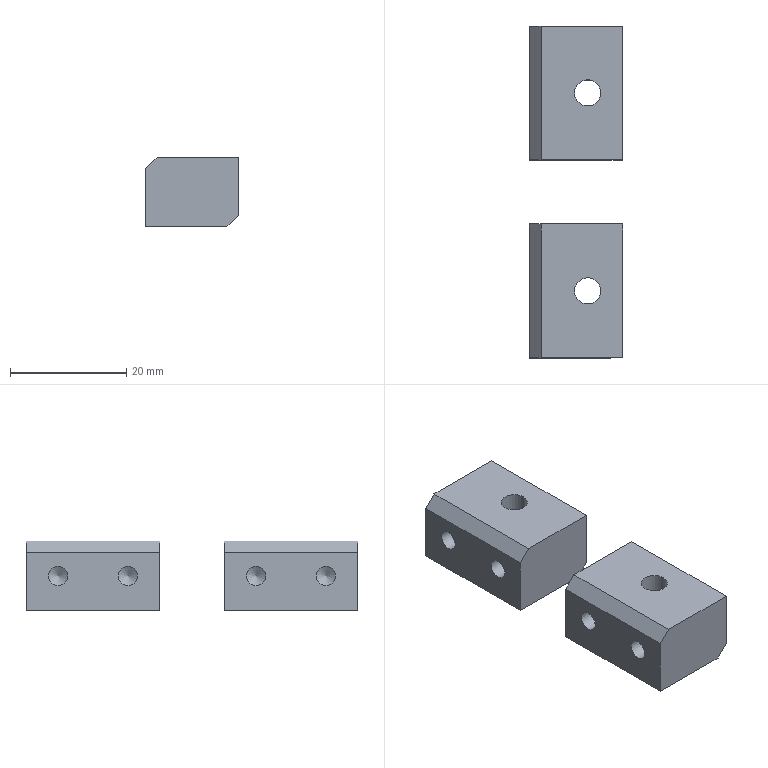Part | NX | 2 solids | 30 faces | box 16 x 57 x 12 mm | volume 7634 mm3 | plane 18 | cylinder 8 | cone 4 | commonest cylinder face diameters 3.3 x4 4.5 x2 8 x2
STEP:
#1=CARTESIAN_POINT('',(14.,11.5,-12.));
#2=VERTEX_POINT('',#1);
#3=CARTESIAN_POINT('',(10.,11.5,-12.));
#4=DIRECTION('',(0.,0.,-1.));
#5=DIRECTION('',(-1.,0.,0.));
#6=AXIS2_PLACEMENT_3D('',#3,#4,#5);
#7=CIRCLE('',#6,4.);
#8=EDGE_CURVE('',#2,#2,#7,.T.);
#9=ORIENTED_EDGE('',*,*,#8,.T.);
#10=EDGE_LOOP('',(#9));
#11=FACE_BOUND('',#10,.T.);
#12=CARTESIAN_POINT('',(6.,11.5,-7.));
#13=VERTEX_POINT('',#12);
#14=CARTESIAN_POINT('',(10.,11.5,-7.));
#15=DIRECTION('',(0.,0.,-1.));
#16=DIRECTION('',(-1.,0.,0.));
#17=AXIS2_PLACEMENT_3D('',#14,#15,#16);
#18=CIRCLE('',#17,4.);
#19=EDGE_CURVE('',#13,#13,#18,.T.);
#20=ORIENTED_EDGE('',*,*,#19,.F.);
#21=EDGE_LOOP('',(#20));
#22=FACE_BOUND('',#21,.T.);
#23=CARTESIAN_POINT('',(10.,11.5,-12.));
#24=DIRECTION('',(0.,0.,-1.));
#25=DIRECTION('',(-1.,0.,0.));
#26=AXIS2_PLACEMENT_3D('',#23,#24,#25);
#27=CYLINDRICAL_SURFACE('',#26,4.);
#28=ADVANCED_FACE('',(#11,#22),#27,.F.);
#29=ORIENTED_EDGE('',*,*,#19,.T.);
#30=EDGE_LOOP('',(#29));
#31=FACE_BOUND('',#30,.T.);
#32=CARTESIAN_POINT('',(7.75,11.5,-7.));
#33=VERTEX_POINT('',#32);
#34=CARTESIAN_POINT('',(10.,11.5,-7.));
#35=DIRECTION('',(0.,0.,-1.));
#36=DIRECTION('',(-1.,0.,0.));
#37=AXIS2_PLACEMENT_3D('',#34,#35,#36);
#38=CIRCLE('',#37,2.25);
#39=EDGE_CURVE('',#33,#33,#38,.T.);
#40=ORIENTED_EDGE('',*,*,#39,.F.);
#41=EDGE_LOOP('',(#40));
#42=FACE_BOUND('',#41,.T.);
#43=CARTESIAN_POINT('',(12.25,11.5,-7.));
#44=DIRECTION('',(0.,0.,1.));
#45=DIRECTION('',(1.,0.,0.));
#46=AXIS2_PLACEMENT_3D('',#43,#44,#45);
#47=PLANE('',#46);
#48=ADVANCED_FACE('',(#31,#42),#47,.F.);
#49=ORIENTED_EDGE('',*,*,#39,.T.);
#50=EDGE_LOOP('',(#49));
#51=FACE_BOUND('',#50,.T.);
#52=CARTESIAN_POINT('',(7.75,11.5,0.));
#53=VERTEX_POINT('',#52);
#54=CARTESIAN_POINT('',(10.,11.5,0.));
#55=DIRECTION('',(0.,0.,-1.));
#56=DIRECTION('',(-1.,0.,0.));
#57=AXIS2_PLACEMENT_3D('',#54,#55,#56);
#58=CIRCLE('',#57,2.25);
#59=EDGE_CURVE('',#53,#53,#58,.T.);
#60=ORIENTED_EDGE('',*,*,#59,.F.);
#61=EDGE_LOOP('',(#60));
#62=FACE_BOUND('',#61,.T.);
#63=CARTESIAN_POINT('',(10.,11.5,-12.));
#64=DIRECTION('',(0.,0.,-1.));
#65=DIRECTION('',(-1.,0.,0.));
#66=AXIS2_PLACEMENT_3D('',#63,#64,#65);
#67=CYLINDRICAL_SURFACE('',#66,2.25);
#68=ADVANCED_FACE('',(#51,#62),#67,.F.);
#69=CARTESIAN_POINT('',(0.,5.5,-4.35));
#70=VERTEX_POINT('',#69);
#71=CARTESIAN_POINT('',(0.,5.5,-6.));
#72=DIRECTION('',(-1.,0.,0.));
#73=DIRECTION('',(0.,0.,1.));
#74=AXIS2_PLACEMENT_3D('',#71,#72,#73);
#75=CIRCLE('',#74,1.65);
#76=EDGE_CURVE('',#70,#70,#75,.T.);
#77=ORIENTED_EDGE('',*,*,#76,.T.);
#78=EDGE_LOOP('',(#77));
#79=FACE_BOUND('',#78,.T.);
#80=CARTESIAN_POINT('',(8.1,5.5,-4.35));
#81=VERTEX_POINT('',#80);
#82=CARTESIAN_POINT('',(8.1,5.5,-6.));
#83=DIRECTION('',(-1.,0.,0.));
#84=DIRECTION('',(0.,0.,1.));
#85=AXIS2_PLACEMENT_3D('',#82,#83,#84);
#86=CIRCLE('',#85,1.65);
#87=EDGE_CURVE('',#81,#81,#86,.T.);
#88=ORIENTED_EDGE('',*,*,#87,.F.);
#89=EDGE_LOOP('',(#88));
#90=FACE_BOUND('',#89,.T.);
#91=CARTESIAN_POINT('',(0.,5.5,-6.));
#92=DIRECTION('',(-1.,0.,0.));
#93=DIRECTION('',(0.,0.,1.));
#94=AXIS2_PLACEMENT_3D('',#91,#92,#93);
#95=CYLINDRICAL_SURFACE('',#94,1.65);
#96=ADVANCED_FACE('',(#79,#90),#95,.F.);
#97=CARTESIAN_POINT('',(9.091,5.5,-6.));
#98=VERTEX_POINT('',#97);
#99=VERTEX_LOOP('',#98);
#100=FACE_BOUND('',#99,.T.);
#101=ORIENTED_EDGE('',*,*,#87,.T.);
#102=EDGE_LOOP('',(#101));
#103=FACE_BOUND('',#102,.T.);
#104=CARTESIAN_POINT('',(8.1,5.5,-6.));
#105=DIRECTION('',(-1.,0.,0.));
#106=DIRECTION('',(0.,0.,1.));
#107=AXIS2_PLACEMENT_3D('',#104,#105,#106);
#108=CONICAL_SURFACE('',#107,1.65,1.03);
#109=ADVANCED_FACE('',(#100,#103),#108,.F.);
#110=CARTESIAN_POINT('',(0.,17.5,-4.35));
#111=VERTEX_POINT('',#110);
#112=CARTESIAN_POINT('',(0.,17.5,-6.));
#113=DIRECTION('',(-1.,0.,0.));
#114=DIRECTION('',(0.,0.,1.));
#115=AXIS2_PLACEMENT_3D('',#112,#113,#114);
#116=CIRCLE('',#115,1.65);
#117=EDGE_CURVE('',#111,#111,#116,.T.);
#118=ORIENTED_EDGE('',*,*,#117,.T.);
#119=EDGE_LOOP('',(#118));
#120=FACE_BOUND('',#119,.T.);
#121=CARTESIAN_POINT('',(8.1,17.5,-4.35));
#122=VERTEX_POINT('',#121);
#123=CARTESIAN_POINT('',(8.1,17.5,-6.));
#124=DIRECTION('',(-1.,0.,0.));
#125=DIRECTION('',(0.,0.,1.));
#126=AXIS2_PLACEMENT_3D('',#123,#124,#125);
#127=CIRCLE('',#126,1.65);
#128=EDGE_CURVE('',#122,#122,#127,.T.);
#129=ORIENTED_EDGE('',*,*,#128,.F.);
#130=EDGE_LOOP('',(#129));
#131=FACE_BOUND('',#130,.T.);
#132=CARTESIAN_POINT('',(0.,17.5,-6.));
#133=DIRECTION('',(-1.,0.,0.));
#134=DIRECTION('',(0.,0.,1.));
#135=AXIS2_PLACEMENT_3D('',#132,#133,#134);
#136=CYLINDRICAL_SURFACE('',#135,1.65);
#137=ADVANCED_FACE('',(#120,#131),#136,.F.);
#138=CARTESIAN_POINT('',(9.091,17.5,-6.));
#139=VERTEX_POINT('',#138);
#140=VERTEX_LOOP('',#139);
#141=FACE_BOUND('',#140,.T.);
#142=ORIENTED_EDGE('',*,*,#128,.T.);
#143=EDGE_LOOP('',(#142));
#144=FACE_BOUND('',#143,.T.);
#145=CARTESIAN_POINT('',(8.1,17.5,-6.));
#146=DIRECTION('',(-1.,0.,0.));
#147=DIRECTION('',(0.,0.,1.));
#148=AXIS2_PLACEMENT_3D('',#145,#146,#147);
#149=CONICAL_SURFACE('',#148,1.65,1.03);
#150=ADVANCED_FACE('',(#141,#144),#149,.F.);
#151=CARTESIAN_POINT('',(0.,23.,-2.));
#152=VERTEX_POINT('',#151);
#153=CARTESIAN_POINT('',(2.,23.,0.));
#154=VERTEX_POINT('',#153);
#155=CARTESIAN_POINT('',(1.,23.,-1.));
#156=DIRECTION('',(0.7071,0.,0.7071));
#157=VECTOR('',#156,1000.);
#158=LINE('',#155,#157);
#159=EDGE_CURVE('',#152,#154,#158,.T.);
#160=ORIENTED_EDGE('',*,*,#159,.F.);
#161=CARTESIAN_POINT('',(0.,0.,-2.));
#162=VERTEX_POINT('',#161);
#163=CARTESIAN_POINT('',(0.,23.,-2.));
#164=DIRECTION('',(0.,1.,0.));
#165=VECTOR('',#164,1000.);
#166=LINE('',#163,#165);
#167=EDGE_CURVE('',#162,#152,#166,.T.);
#168=ORIENTED_EDGE('',*,*,#167,.F.);
#169=CARTESIAN_POINT('',(2.,0.,0.));
#170=VERTEX_POINT('',#169);
#171=CARTESIAN_POINT('',(2.,0.,0.));
#172=DIRECTION('',(-0.7071,0.,-0.7071));
#173=VECTOR('',#172,1000.);
#174=LINE('',#171,#173);
#175=EDGE_CURVE('',#170,#162,#174,.T.);
#176=ORIENTED_EDGE('',*,*,#175,.F.);
#177=CARTESIAN_POINT('',(2.,23.,0.));
#178=DIRECTION('',(0.,-1.,0.));
#179=VECTOR('',#178,1000.);
#180=LINE('',#177,#179);
#181=EDGE_CURVE('',#154,#170,#180,.T.);
#182=ORIENTED_EDGE('',*,*,#181,.F.);
#183=EDGE_LOOP('',(#160,#168,#176,#182));
#184=FACE_BOUND('',#183,.T.);
#185=CARTESIAN_POINT('',(2.,23.,0.));
#186=DIRECTION('',(0.7071,0.,-0.7071));
#187=DIRECTION('',(0.,-1.,0.));
#188=AXIS2_PLACEMENT_3D('',#185,#186,#187);
#189=PLANE('',#188);
#190=ADVANCED_FACE('',(#184),#189,.F.);
#191=CARTESIAN_POINT('',(16.,23.,-10.));
#192=VERTEX_POINT('',#191);
#193=CARTESIAN_POINT('',(14.,23.,-12.));
#194=VERTEX_POINT('',#193);
#195=CARTESIAN_POINT('',(13.,23.,-13.));
#196=DIRECTION('',(-0.7071,0.,-0.7071));
#197=VECTOR('',#196,1000.);
#198=LINE('',#195,#197);
#199=EDGE_CURVE('',#192,#194,#198,.T.);
#200=ORIENTED_EDGE('',*,*,#199,.F.);
#201=CARTESIAN_POINT('',(16.,0.,-10.));
#202=VERTEX_POINT('',#201);
#203=CARTESIAN_POINT('',(16.,23.,-10.));
#204=DIRECTION('',(0.,1.,0.));
#205=VECTOR('',#204,1000.);
#206=LINE('',#203,#205);
#207=EDGE_CURVE('',#202,#192,#206,.T.);
#208=ORIENTED_EDGE('',*,*,#207,.F.);
#209=CARTESIAN_POINT('',(14.,0.,-12.));
#210=VERTEX_POINT('',#209);
#211=CARTESIAN_POINT('',(14.,0.,-12.));
#212=DIRECTION('',(0.7071,0.,0.7071));
#213=VECTOR('',#212,1000.);
#214=LINE('',#211,#213);
#215=EDGE_CURVE('',#210,#202,#214,.T.);
#216=ORIENTED_EDGE('',*,*,#215,.F.);
#217=CARTESIAN_POINT('',(14.,23.,-12.));
#218=DIRECTION('',(0.,-1.,0.));
#219=VECTOR('',#218,1000.);
#220=LINE('',#217,#219);
#221=EDGE_CURVE('',#2,#210,#220,.T.);
#222=ORIENTED_EDGE('',*,*,#221,.F.);
#223=CARTESIAN_POINT('',(14.,23.,-12.));
#224=DIRECTION('',(0.,-1.,0.));
#225=VECTOR('',#224,1000.);
#226=LINE('',#223,#225);
#227=EDGE_CURVE('',#194,#2,#226,.T.);
#228=ORIENTED_EDGE('',*,*,#227,.F.);
#229=EDGE_LOOP('',(#200,#208,#216,#222,#228));
#230=FACE_BOUND('',#229,.T.);
#231=CARTESIAN_POINT('',(14.,23.,-12.));
#232=DIRECTION('',(-0.7071,0.,0.7071));
#233=DIRECTION('',(0.,-1.,0.));
#234=AXIS2_PLACEMENT_3D('',#231,#232,#233);
#235=PLANE('',#234);
#236=ADVANCED_FACE('',(#230),#235,.F.);
#237=CARTESIAN_POINT('',(0.,0.,-12.));
#238=VERTEX_POINT('',#237);
#239=CARTESIAN_POINT('',(16.,0.,-12.));
#240=DIRECTION('',(-1.,0.,0.));
#241=VECTOR('',#240,1000.);
#242=LINE('',#239,#241);
#243=EDGE_CURVE('',#210,#238,#242,.T.);
#244=ORIENTED_EDGE('',*,*,#243,.F.);
#245=ORIENTED_EDGE('',*,*,#215,.T.);
#246=CARTESIAN_POINT('',(16.,0.,0.));
#247=VERTEX_POINT('',#246);
#248=CARTESIAN_POINT('',(16.,0.,0.));
#249=DIRECTION('',(0.,0.,-1.));
#250=VECTOR('',#249,1000.);
#251=LINE('',#248,#250);
#252=EDGE_CURVE('',#247,#202,#251,.T.);
#253=ORIENTED_EDGE('',*,*,#252,.F.);
#254=CARTESIAN_POINT('',(0.,0.,0.));
#255=DIRECTION('',(1.,0.,0.));
#256=VECTOR('',#255,1000.);
#257=LINE('',#254,#256);
#258=EDGE_CURVE('',#170,#247,#257,.T.);
#259=ORIENTED_EDGE('',*,*,#258,.F.);
#260=ORIENTED_EDGE('',*,*,#175,.T.);
#261=CARTESIAN_POINT('',(0.,0.,-12.));
#262=DIRECTION('',(0.,0.,1.));
#263=VECTOR('',#262,1000.);
#264=LINE('',#261,#263);
#265=EDGE_CURVE('',#238,#162,#264,.T.);
#266=ORIENTED_EDGE('',*,*,#265,.F.);
#267=EDGE_LOOP('',(#244,#245,#253,#259,#260,#266));
#268=FACE_BOUND('',#267,.T.);
#269=CARTESIAN_POINT('',(0.,0.,0.));
#270=DIRECTION('',(0.,1.,0.));
#271=DIRECTION('',(0.,0.,1.));
#272=AXIS2_PLACEMENT_3D('',#269,#270,#271);
#273=PLANE('',#272);
#274=ADVANCED_FACE('',(#268),#273,.F.);
#275=CARTESIAN_POINT('',(16.,23.,0.));
#276=VERTEX_POINT('',#275);
#277=CARTESIAN_POINT('',(16.,23.,0.));
#278=DIRECTION('',(0.,0.,-1.));
#279=VECTOR('',#278,1000.);
#280=LINE('',#277,#279);
#281=EDGE_CURVE('',#276,#192,#280,.T.);
#282=ORIENTED_EDGE('',*,*,#281,.T.);
#283=ORIENTED_EDGE('',*,*,#199,.T.);
#284=CARTESIAN_POINT('',(0.,23.,-12.));
#285=VERTEX_POINT('',#284);
#286=CARTESIAN_POINT('',(16.,23.,-12.));
#287=DIRECTION('',(-1.,0.,0.));
#288=VECTOR('',#287,1000.);
#289=LINE('',#286,#288);
#290=EDGE_CURVE('',#194,#285,#289,.T.);
#291=ORIENTED_EDGE('',*,*,#290,.T.);
#292=CARTESIAN_POINT('',(0.,23.,-12.));
#293=DIRECTION('',(0.,0.,1.));
#294=VECTOR('',#293,1000.);
#295=LINE('',#292,#294);
#296=EDGE_CURVE('',#285,#152,#295,.T.);
#297=ORIENTED_EDGE('',*,*,#296,.T.);
#298=ORIENTED_EDGE('',*,*,#159,.T.);
#299=CARTESIAN_POINT('',(0.,23.,0.));
#300=DIRECTION('',(1.,0.,0.));
#301=VECTOR('',#300,1000.);
#302=LINE('',#299,#301);
#303=EDGE_CURVE('',#154,#276,#302,.T.);
#304=ORIENTED_EDGE('',*,*,#303,.T.);
#305=EDGE_LOOP('',(#282,#283,#291,#297,#298,#304));
#306=FACE_BOUND('',#305,.T.);
#307=CARTESIAN_POINT('',(0.,23.,0.));
#308=DIRECTION('',(0.,1.,0.));
#309=DIRECTION('',(0.,0.,1.));
#310=AXIS2_PLACEMENT_3D('',#307,#308,#309);
#311=PLANE('',#310);
#312=ADVANCED_FACE('',(#306),#311,.T.);
#313=ORIENTED_EDGE('',*,*,#252,.T.);
#314=ORIENTED_EDGE('',*,*,#207,.T.);
#315=ORIENTED_EDGE('',*,*,#281,.F.);
#316=CARTESIAN_POINT('',(16.,23.,0.));
#317=DIRECTION('',(0.,-1.,0.));
#318=VECTOR('',#317,1000.);
#319=LINE('',#316,#318);
#320=EDGE_CURVE('',#276,#247,#319,.T.);
#321=ORIENTED_EDGE('',*,*,#320,.T.);
#322=EDGE_LOOP('',(#313,#314,#315,#321));
#323=FACE_BOUND('',#322,.T.);
#324=CARTESIAN_POINT('',(16.,23.,0.));
#325=DIRECTION('',(-1.,0.,0.));
#326=DIRECTION('',(0.,0.,1.));
#327=AXIS2_PLACEMENT_3D('',#324,#325,#326);
#328=PLANE('',#327);
#329=ADVANCED_FACE('',(#323),#328,.F.);
#330=ORIENTED_EDGE('',*,*,#303,.F.);
#331=ORIENTED_EDGE('',*,*,#181,.T.);
#332=ORIENTED_EDGE('',*,*,#258,.T.);
#333=ORIENTED_EDGE('',*,*,#320,.F.);
#334=EDGE_LOOP('',(#330,#331,#332,#333));
#335=FACE_BOUND('',#334,.T.);
#336=ORIENTED_EDGE('',*,*,#59,.T.);
#337=EDGE_LOOP('',(#336));
#338=FACE_BOUND('',#337,.T.);
#339=CARTESIAN_POINT('',(0.,23.,0.));
#340=DIRECTION('',(0.,0.,-1.));
#341=DIRECTION('',(-1.,0.,0.));
#342=AXIS2_PLACEMENT_3D('',#339,#340,#341);
#343=PLANE('',#342);
#344=ADVANCED_FACE('',(#335,#338),#343,.F.);
#345=ORIENTED_EDGE('',*,*,#265,.T.);
#346=ORIENTED_EDGE('',*,*,#167,.T.);
#347=ORIENTED_EDGE('',*,*,#296,.F.);
#348=CARTESIAN_POINT('',(0.,23.,-12.));
#349=DIRECTION('',(0.,-1.,0.));
#350=VECTOR('',#349,1000.);
#351=LINE('',#348,#350);
#352=EDGE_CURVE('',#285,#238,#351,.T.);
#353=ORIENTED_EDGE('',*,*,#352,.T.);
#354=EDGE_LOOP('',(#345,#346,#347,#353));
#355=FACE_BOUND('',#354,.T.);
#356=ORIENTED_EDGE('',*,*,#117,.F.);
#357=EDGE_LOOP('',(#356));
#358=FACE_BOUND('',#357,.T.);
#359=ORIENTED_EDGE('',*,*,#76,.F.);
#360=EDGE_LOOP('',(#359));
#361=FACE_BOUND('',#360,.T.);
#362=CARTESIAN_POINT('',(0.,23.,-12.));
#363=DIRECTION('',(1.,0.,0.));
#364=DIRECTION('',(0.,0.,-1.));
#365=AXIS2_PLACEMENT_3D('',#362,#363,#364);
#366=PLANE('',#365);
#367=ADVANCED_FACE('',(#355,#358,#361),#366,.F.);
#368=ORIENTED_EDGE('',*,*,#227,.T.);
#369=ORIENTED_EDGE('',*,*,#8,.F.);
#370=ORIENTED_EDGE('',*,*,#221,.T.);
#371=ORIENTED_EDGE('',*,*,#243,.T.);
#372=ORIENTED_EDGE('',*,*,#352,.F.);
#373=ORIENTED_EDGE('',*,*,#290,.F.);
#374=EDGE_LOOP('',(#368,#369,#370,#371,#372,#373));
#375=FACE_BOUND('',#374,.T.);
#376=CARTESIAN_POINT('',(16.,23.,-12.));
#377=DIRECTION('',(0.,0.,1.));
#378=DIRECTION('',(1.,0.,0.));
#379=AXIS2_PLACEMENT_3D('',#376,#377,#378);
#380=PLANE('',#379);
#381=ADVANCED_FACE('',(#375),#380,.F.);
#382=CLOSED_SHELL('',(#28,#48,#68,#96,#109,#137,#150,#190,#236,#274,#312,#329,#344,#367,#381));
#383=MANIFOLD_SOLID_BREP('',#382);
#384=CARTESIAN_POINT('',(14.,45.5,-12.));
#385=VERTEX_POINT('',#384);
#386=CARTESIAN_POINT('',(10.,45.5,-12.));
#387=DIRECTION('',(0.,0.,-1.));
#388=DIRECTION('',(-1.,0.,0.));
#389=AXIS2_PLACEMENT_3D('',#386,#387,#388);
#390=CIRCLE('',#389,4.);
#391=EDGE_CURVE('',#385,#385,#390,.T.);
#392=ORIENTED_EDGE('',*,*,#391,.T.);
#393=EDGE_LOOP('',(#392));
#394=FACE_BOUND('',#393,.T.);
#395=CARTESIAN_POINT('',(6.,45.5,-7.));
#396=VERTEX_POINT('',#395);
#397=CARTESIAN_POINT('',(10.,45.5,-7.));
#398=DIRECTION('',(0.,0.,-1.));
#399=DIRECTION('',(-1.,0.,0.));
#400=AXIS2_PLACEMENT_3D('',#397,#398,#399);
#401=CIRCLE('',#400,4.);
#402=EDGE_CURVE('',#396,#396,#401,.T.);
#403=ORIENTED_EDGE('',*,*,#402,.F.);
#404=EDGE_LOOP('',(#403));
#405=FACE_BOUND('',#404,.T.);
#406=CARTESIAN_POINT('',(10.,45.5,-12.));
#407=DIRECTION('',(0.,0.,-1.));
#408=DIRECTION('',(-1.,0.,0.));
#409=AXIS2_PLACEMENT_3D('',#406,#407,#408);
#410=CYLINDRICAL_SURFACE('',#409,4.);
#411=ADVANCED_FACE('',(#394,#405),#410,.F.);
#412=ORIENTED_EDGE('',*,*,#402,.T.);
#413=EDGE_LOOP('',(#412));
#414=FACE_BOUND('',#413,.T.);
#415=CARTESIAN_POINT('',(7.75,45.5,-7.));
#416=VERTEX_POINT('',#415);
#417=CARTESIAN_POINT('',(10.,45.5,-7.));
#418=DIRECTION('',(0.,0.,-1.));
#419=DIRECTION('',(-1.,0.,0.));
#420=AXIS2_PLACEMENT_3D('',#417,#418,#419);
#421=CIRCLE('',#420,2.25);
#422=EDGE_CURVE('',#416,#416,#421,.T.);
#423=ORIENTED_EDGE('',*,*,#422,.F.);
#424=EDGE_LOOP('',(#423));
#425=FACE_BOUND('',#424,.T.);
#426=CARTESIAN_POINT('',(12.25,45.5,-7.));
#427=DIRECTION('',(0.,0.,1.));
#428=DIRECTION('',(1.,0.,0.));
#429=AXIS2_PLACEMENT_3D('',#426,#427,#428);
#430=PLANE('',#429);
#431=ADVANCED_FACE('',(#414,#425),#430,.F.);
#432=ORIENTED_EDGE('',*,*,#422,.T.);
#433=EDGE_LOOP('',(#432));
#434=FACE_BOUND('',#433,.T.);
#435=CARTESIAN_POINT('',(7.75,45.5,0.));
#436=VERTEX_POINT('',#435);
#437=CARTESIAN_POINT('',(10.,45.5,0.));
#438=DIRECTION('',(0.,0.,-1.));
#439=DIRECTION('',(-1.,0.,0.));
#440=AXIS2_PLACEMENT_3D('',#437,#438,#439);
#441=CIRCLE('',#440,2.25);
#442=EDGE_CURVE('',#436,#436,#441,.T.);
#443=ORIENTED_EDGE('',*,*,#442,.F.);
#444=EDGE_LOOP('',(#443));
#445=FACE_BOUND('',#444,.T.);
#446=CARTESIAN_POINT('',(10.,45.5,-12.));
#447=DIRECTION('',(0.,0.,-1.));
#448=DIRECTION('',(-1.,0.,0.));
#449=AXIS2_PLACEMENT_3D('',#446,#447,#448);
#450=CYLINDRICAL_SURFACE('',#449,2.25);
#451=ADVANCED_FACE('',(#434,#445),#450,.F.);
#452=CARTESIAN_POINT('',(0.,39.5,-4.35));
#453=VERTEX_POINT('',#452);
#454=CARTESIAN_POINT('',(0.,39.5,-6.));
#455=DIRECTION('',(-1.,0.,0.));
#456=DIRECTION('',(0.,0.,1.));
#457=AXIS2_PLACEMENT_3D('',#454,#455,#456);
#458=CIRCLE('',#457,1.65);
#459=EDGE_CURVE('',#453,#453,#458,.T.);
#460=ORIENTED_EDGE('',*,*,#459,.T.);
#461=EDGE_LOOP('',(#460));
#462=FACE_BOUND('',#461,.T.);
#463=CARTESIAN_POINT('',(8.1,39.5,-4.35));
#464=VERTEX_POINT('',#463);
#465=CARTESIAN_POINT('',(8.1,39.5,-6.));
#466=DIRECTION('',(-1.,0.,0.));
#467=DIRECTION('',(0.,0.,1.));
#468=AXIS2_PLACEMENT_3D('',#465,#466,#467);
#469=CIRCLE('',#468,1.65);
#470=EDGE_CURVE('',#464,#464,#469,.T.);
#471=ORIENTED_EDGE('',*,*,#470,.F.);
#472=EDGE_LOOP('',(#471));
#473=FACE_BOUND('',#472,.T.);
#474=CARTESIAN_POINT('',(0.,39.5,-6.));
#475=DIRECTION('',(-1.,0.,0.));
#476=DIRECTION('',(0.,0.,1.));
#477=AXIS2_PLACEMENT_3D('',#474,#475,#476);
#478=CYLINDRICAL_SURFACE('',#477,1.65);
#479=ADVANCED_FACE('',(#462,#473),#478,.F.);
#480=CARTESIAN_POINT('',(9.091,39.5,-6.));
#481=VERTEX_POINT('',#480);
#482=VERTEX_LOOP('',#481);
#483=FACE_BOUND('',#482,.T.);
#484=ORIENTED_EDGE('',*,*,#470,.T.);
#485=EDGE_LOOP('',(#484));
#486=FACE_BOUND('',#485,.T.);
#487=CARTESIAN_POINT('',(8.1,39.5,-6.));
#488=DIRECTION('',(-1.,0.,0.));
#489=DIRECTION('',(0.,0.,1.));
#490=AXIS2_PLACEMENT_3D('',#487,#488,#489);
#491=CONICAL_SURFACE('',#490,1.65,1.03);
#492=ADVANCED_FACE('',(#483,#486),#491,.F.);
#493=CARTESIAN_POINT('',(0.,51.5,-4.35));
#494=VERTEX_POINT('',#493);
#495=CARTESIAN_POINT('',(0.,51.5,-6.));
#496=DIRECTION('',(-1.,0.,0.));
#497=DIRECTION('',(0.,0.,1.));
#498=AXIS2_PLACEMENT_3D('',#495,#496,#497);
#499=CIRCLE('',#498,1.65);
#500=EDGE_CURVE('',#494,#494,#499,.T.);
#501=ORIENTED_EDGE('',*,*,#500,.T.);
#502=EDGE_LOOP('',(#501));
#503=FACE_BOUND('',#502,.T.);
#504=CARTESIAN_POINT('',(8.1,51.5,-4.35));
#505=VERTEX_POINT('',#504);
#506=CARTESIAN_POINT('',(8.1,51.5,-6.));
#507=DIRECTION('',(-1.,0.,0.));
#508=DIRECTION('',(0.,0.,1.));
#509=AXIS2_PLACEMENT_3D('',#506,#507,#508);
#510=CIRCLE('',#509,1.65);
#511=EDGE_CURVE('',#505,#505,#510,.T.);
#512=ORIENTED_EDGE('',*,*,#511,.F.);
#513=EDGE_LOOP('',(#512));
#514=FACE_BOUND('',#513,.T.);
#515=CARTESIAN_POINT('',(0.,51.5,-6.));
#516=DIRECTION('',(-1.,0.,0.));
#517=DIRECTION('',(0.,0.,1.));
#518=AXIS2_PLACEMENT_3D('',#515,#516,#517);
#519=CYLINDRICAL_SURFACE('',#518,1.65);
#520=ADVANCED_FACE('',(#503,#514),#519,.F.);
#521=CARTESIAN_POINT('',(9.091,51.5,-6.));
#522=VERTEX_POINT('',#521);
#523=VERTEX_LOOP('',#522);
#524=FACE_BOUND('',#523,.T.);
#525=ORIENTED_EDGE('',*,*,#511,.T.);
#526=EDGE_LOOP('',(#525));
#527=FACE_BOUND('',#526,.T.);
#528=CARTESIAN_POINT('',(8.1,51.5,-6.));
#529=DIRECTION('',(-1.,0.,0.));
#530=DIRECTION('',(0.,0.,1.));
#531=AXIS2_PLACEMENT_3D('',#528,#529,#530);
#532=CONICAL_SURFACE('',#531,1.65,1.03);
#533=ADVANCED_FACE('',(#524,#527),#532,.F.);
#534=CARTESIAN_POINT('',(0.,57.,-2.));
#535=VERTEX_POINT('',#534);
#536=CARTESIAN_POINT('',(2.,57.,0.));
#537=VERTEX_POINT('',#536);
#538=CARTESIAN_POINT('',(1.,57.,-1.));
#539=DIRECTION('',(0.7071,0.,0.7071));
#540=VECTOR('',#539,1000.);
#541=LINE('',#538,#540);
#542=EDGE_CURVE('',#535,#537,#541,.T.);
#543=ORIENTED_EDGE('',*,*,#542,.F.);
#544=CARTESIAN_POINT('',(0.,34.,-2.));
#545=VERTEX_POINT('',#544);
#546=CARTESIAN_POINT('',(0.,57.,-2.));
#547=DIRECTION('',(0.,1.,0.));
#548=VECTOR('',#547,1000.);
#549=LINE('',#546,#548);
#550=EDGE_CURVE('',#545,#535,#549,.T.);
#551=ORIENTED_EDGE('',*,*,#550,.F.);
#552=CARTESIAN_POINT('',(2.,34.,0.));
#553=VERTEX_POINT('',#552);
#554=CARTESIAN_POINT('',(2.,34.,0.));
#555=DIRECTION('',(-0.7071,0.,-0.7071));
#556=VECTOR('',#555,1000.);
#557=LINE('',#554,#556);
#558=EDGE_CURVE('',#553,#545,#557,.T.);
#559=ORIENTED_EDGE('',*,*,#558,.F.);
#560=CARTESIAN_POINT('',(2.,57.,0.));
#561=DIRECTION('',(0.,-1.,0.));
#562=VECTOR('',#561,1000.);
#563=LINE('',#560,#562);
#564=EDGE_CURVE('',#537,#553,#563,.T.);
#565=ORIENTED_EDGE('',*,*,#564,.F.);
#566=EDGE_LOOP('',(#543,#551,#559,#565));
#567=FACE_BOUND('',#566,.T.);
#568=CARTESIAN_POINT('',(2.,57.,0.));
#569=DIRECTION('',(0.7071,0.,-0.7071));
#570=DIRECTION('',(0.,-1.,0.));
#571=AXIS2_PLACEMENT_3D('',#568,#569,#570);
#572=PLANE('',#571);
#573=ADVANCED_FACE('',(#567),#572,.F.);
#574=CARTESIAN_POINT('',(16.,57.,-10.));
#575=VERTEX_POINT('',#574);
#576=CARTESIAN_POINT('',(14.,57.,-12.));
#577=VERTEX_POINT('',#576);
#578=CARTESIAN_POINT('',(13.,57.,-13.));
#579=DIRECTION('',(-0.7071,0.,-0.7071));
#580=VECTOR('',#579,1000.);
#581=LINE('',#578,#580);
#582=EDGE_CURVE('',#575,#577,#581,.T.);
#583=ORIENTED_EDGE('',*,*,#582,.F.);
#584=CARTESIAN_POINT('',(16.,34.,-10.));
#585=VERTEX_POINT('',#584);
#586=CARTESIAN_POINT('',(16.,57.,-10.));
#587=DIRECTION('',(0.,1.,0.));
#588=VECTOR('',#587,1000.);
#589=LINE('',#586,#588);
#590=EDGE_CURVE('',#585,#575,#589,.T.);
#591=ORIENTED_EDGE('',*,*,#590,.F.);
#592=CARTESIAN_POINT('',(14.,34.,-12.));
#593=VERTEX_POINT('',#592);
#594=CARTESIAN_POINT('',(14.,34.,-12.));
#595=DIRECTION('',(0.7071,0.,0.7071));
#596=VECTOR('',#595,1000.);
#597=LINE('',#594,#596);
#598=EDGE_CURVE('',#593,#585,#597,.T.);
#599=ORIENTED_EDGE('',*,*,#598,.F.);
#600=CARTESIAN_POINT('',(14.,57.,-12.));
#601=DIRECTION('',(0.,-1.,0.));
#602=VECTOR('',#601,1000.);
#603=LINE('',#600,#602);
#604=EDGE_CURVE('',#385,#593,#603,.T.);
#605=ORIENTED_EDGE('',*,*,#604,.F.);
#606=CARTESIAN_POINT('',(14.,57.,-12.));
#607=DIRECTION('',(0.,-1.,0.));
#608=VECTOR('',#607,1000.);
#609=LINE('',#606,#608);
#610=EDGE_CURVE('',#577,#385,#609,.T.);
#611=ORIENTED_EDGE('',*,*,#610,.F.);
#612=EDGE_LOOP('',(#583,#591,#599,#605,#611));
#613=FACE_BOUND('',#612,.T.);
#614=CARTESIAN_POINT('',(14.,57.,-12.));
#615=DIRECTION('',(-0.7071,0.,0.7071));
#616=DIRECTION('',(0.,-1.,0.));
#617=AXIS2_PLACEMENT_3D('',#614,#615,#616);
#618=PLANE('',#617);
#619=ADVANCED_FACE('',(#613),#618,.F.);
#620=CARTESIAN_POINT('',(0.,34.,-12.));
#621=VERTEX_POINT('',#620);
#622=CARTESIAN_POINT('',(16.,34.,-12.));
#623=DIRECTION('',(-1.,0.,0.));
#624=VECTOR('',#623,1000.);
#625=LINE('',#622,#624);
#626=EDGE_CURVE('',#593,#621,#625,.T.);
#627=ORIENTED_EDGE('',*,*,#626,.F.);
#628=ORIENTED_EDGE('',*,*,#598,.T.);
#629=CARTESIAN_POINT('',(16.,34.,0.));
#630=VERTEX_POINT('',#629);
#631=CARTESIAN_POINT('',(16.,34.,0.));
#632=DIRECTION('',(0.,0.,-1.));
#633=VECTOR('',#632,1000.);
#634=LINE('',#631,#633);
#635=EDGE_CURVE('',#630,#585,#634,.T.);
#636=ORIENTED_EDGE('',*,*,#635,.F.);
#637=CARTESIAN_POINT('',(0.,34.,0.));
#638=DIRECTION('',(1.,0.,0.));
#639=VECTOR('',#638,1000.);
#640=LINE('',#637,#639);
#641=EDGE_CURVE('',#553,#630,#640,.T.);
#642=ORIENTED_EDGE('',*,*,#641,.F.);
#643=ORIENTED_EDGE('',*,*,#558,.T.);
#644=CARTESIAN_POINT('',(0.,34.,-12.));
#645=DIRECTION('',(0.,0.,1.));
#646=VECTOR('',#645,1000.);
#647=LINE('',#644,#646);
#648=EDGE_CURVE('',#621,#545,#647,.T.);
#649=ORIENTED_EDGE('',*,*,#648,.F.);
#650=EDGE_LOOP('',(#627,#628,#636,#642,#643,#649));
#651=FACE_BOUND('',#650,.T.);
#652=CARTESIAN_POINT('',(0.,34.,0.));
#653=DIRECTION('',(0.,1.,0.));
#654=DIRECTION('',(0.,0.,1.));
#655=AXIS2_PLACEMENT_3D('',#652,#653,#654);
#656=PLANE('',#655);
#657=ADVANCED_FACE('',(#651),#656,.F.);
#658=CARTESIAN_POINT('',(16.,57.,0.));
#659=VERTEX_POINT('',#658);
#660=CARTESIAN_POINT('',(16.,57.,0.));
#661=DIRECTION('',(0.,0.,-1.));
#662=VECTOR('',#661,1000.);
#663=LINE('',#660,#662);
#664=EDGE_CURVE('',#659,#575,#663,.T.);
#665=ORIENTED_EDGE('',*,*,#664,.T.);
#666=ORIENTED_EDGE('',*,*,#582,.T.);
#667=CARTESIAN_POINT('',(0.,57.,-12.));
#668=VERTEX_POINT('',#667);
#669=CARTESIAN_POINT('',(16.,57.,-12.));
#670=DIRECTION('',(-1.,0.,0.));
#671=VECTOR('',#670,1000.);
#672=LINE('',#669,#671);
#673=EDGE_CURVE('',#577,#668,#672,.T.);
#674=ORIENTED_EDGE('',*,*,#673,.T.);
#675=CARTESIAN_POINT('',(0.,57.,-12.));
#676=DIRECTION('',(0.,0.,1.));
#677=VECTOR('',#676,1000.);
#678=LINE('',#675,#677);
#679=EDGE_CURVE('',#668,#535,#678,.T.);
#680=ORIENTED_EDGE('',*,*,#679,.T.);
#681=ORIENTED_EDGE('',*,*,#542,.T.);
#682=CARTESIAN_POINT('',(0.,57.,0.));
#683=DIRECTION('',(1.,0.,0.));
#684=VECTOR('',#683,1000.);
#685=LINE('',#682,#684);
#686=EDGE_CURVE('',#537,#659,#685,.T.);
#687=ORIENTED_EDGE('',*,*,#686,.T.);
#688=EDGE_LOOP('',(#665,#666,#674,#680,#681,#687));
#689=FACE_BOUND('',#688,.T.);
#690=CARTESIAN_POINT('',(0.,57.,0.));
#691=DIRECTION('',(0.,1.,0.));
#692=DIRECTION('',(0.,0.,1.));
#693=AXIS2_PLACEMENT_3D('',#690,#691,#692);
#694=PLANE('',#693);
#695=ADVANCED_FACE('',(#689),#694,.T.);
#696=ORIENTED_EDGE('',*,*,#635,.T.);
#697=ORIENTED_EDGE('',*,*,#590,.T.);
#698=ORIENTED_EDGE('',*,*,#664,.F.);
#699=CARTESIAN_POINT('',(16.,57.,0.));
#700=DIRECTION('',(0.,-1.,0.));
#701=VECTOR('',#700,1000.);
#702=LINE('',#699,#701);
#703=EDGE_CURVE('',#659,#630,#702,.T.);
#704=ORIENTED_EDGE('',*,*,#703,.T.);
#705=EDGE_LOOP('',(#696,#697,#698,#704));
#706=FACE_BOUND('',#705,.T.);
#707=CARTESIAN_POINT('',(16.,57.,0.));
#708=DIRECTION('',(-1.,0.,0.));
#709=DIRECTION('',(0.,0.,1.));
#710=AXIS2_PLACEMENT_3D('',#707,#708,#709);
#711=PLANE('',#710);
#712=ADVANCED_FACE('',(#706),#711,.F.);
#713=ORIENTED_EDGE('',*,*,#686,.F.);
#714=ORIENTED_EDGE('',*,*,#564,.T.);
#715=ORIENTED_EDGE('',*,*,#641,.T.);
#716=ORIENTED_EDGE('',*,*,#703,.F.);
#717=EDGE_LOOP('',(#713,#714,#715,#716));
#718=FACE_BOUND('',#717,.T.);
#719=ORIENTED_EDGE('',*,*,#442,.T.);
#720=EDGE_LOOP('',(#719));
#721=FACE_BOUND('',#720,.T.);
#722=CARTESIAN_POINT('',(0.,57.,0.));
#723=DIRECTION('',(0.,0.,-1.));
#724=DIRECTION('',(-1.,0.,0.));
#725=AXIS2_PLACEMENT_3D('',#722,#723,#724);
#726=PLANE('',#725);
#727=ADVANCED_FACE('',(#718,#721),#726,.F.);
#728=ORIENTED_EDGE('',*,*,#648,.T.);
#729=ORIENTED_EDGE('',*,*,#550,.T.);
#730=ORIENTED_EDGE('',*,*,#679,.F.);
#731=CARTESIAN_POINT('',(0.,57.,-12.));
#732=DIRECTION('',(0.,-1.,0.));
#733=VECTOR('',#732,1000.);
#734=LINE('',#731,#733);
#735=EDGE_CURVE('',#668,#621,#734,.T.);
#736=ORIENTED_EDGE('',*,*,#735,.T.);
#737=EDGE_LOOP('',(#728,#729,#730,#736));
#738=FACE_BOUND('',#737,.T.);
#739=ORIENTED_EDGE('',*,*,#500,.F.);
#740=EDGE_LOOP('',(#739));
#741=FACE_BOUND('',#740,.T.);
#742=ORIENTED_EDGE('',*,*,#459,.F.);
#743=EDGE_LOOP('',(#742));
#744=FACE_BOUND('',#743,.T.);
#745=CARTESIAN_POINT('',(0.,57.,-12.));
#746=DIRECTION('',(1.,0.,0.));
#747=DIRECTION('',(0.,0.,-1.));
#748=AXIS2_PLACEMENT_3D('',#745,#746,#747);
#749=PLANE('',#748);
#750=ADVANCED_FACE('',(#738,#741,#744),#749,.F.);
#751=ORIENTED_EDGE('',*,*,#610,.T.);
#752=ORIENTED_EDGE('',*,*,#391,.F.);
#753=ORIENTED_EDGE('',*,*,#604,.T.);
#754=ORIENTED_EDGE('',*,*,#626,.T.);
#755=ORIENTED_EDGE('',*,*,#735,.F.);
#756=ORIENTED_EDGE('',*,*,#673,.F.);
#757=EDGE_LOOP('',(#751,#752,#753,#754,#755,#756));
#758=FACE_BOUND('',#757,.T.);
#759=CARTESIAN_POINT('',(16.,57.,-12.));
#760=DIRECTION('',(0.,0.,1.));
#761=DIRECTION('',(1.,0.,0.));
#762=AXIS2_PLACEMENT_3D('',#759,#760,#761);
#763=PLANE('',#762);
#764=ADVANCED_FACE('',(#758),#763,.F.);
#765=CLOSED_SHELL('',(#411,#431,#451,#479,#492,#520,#533,#573,#619,#657,#695,#712,#727,#750,#764));
#766=MANIFOLD_SOLID_BREP('',#765);
#767=(LENGTH_UNIT()NAMED_UNIT(*)SI_UNIT(.MILLI.,.METRE.));
#768=UNCERTAINTY_MEASURE_WITH_UNIT(LENGTH_MEASURE(0.00001),#767,'','');
#769=(NAMED_UNIT(*)PLANE_ANGLE_UNIT()SI_UNIT($,.RADIAN.));
#770=(NAMED_UNIT(*)SI_UNIT($,.STERADIAN.)SOLID_ANGLE_UNIT());
#771=(GEOMETRIC_REPRESENTATION_CONTEXT(3)GLOBAL_UNCERTAINTY_ASSIGNED_CONTEXT((#768))GLOBAL_UNIT_ASSIGNED_CONTEXT((#767,#769,#770))REPRESENTATION_CONTEXT('',''));
#772=ADVANCED_BREP_SHAPE_REPRESENTATION('',(#383,#766),#771);